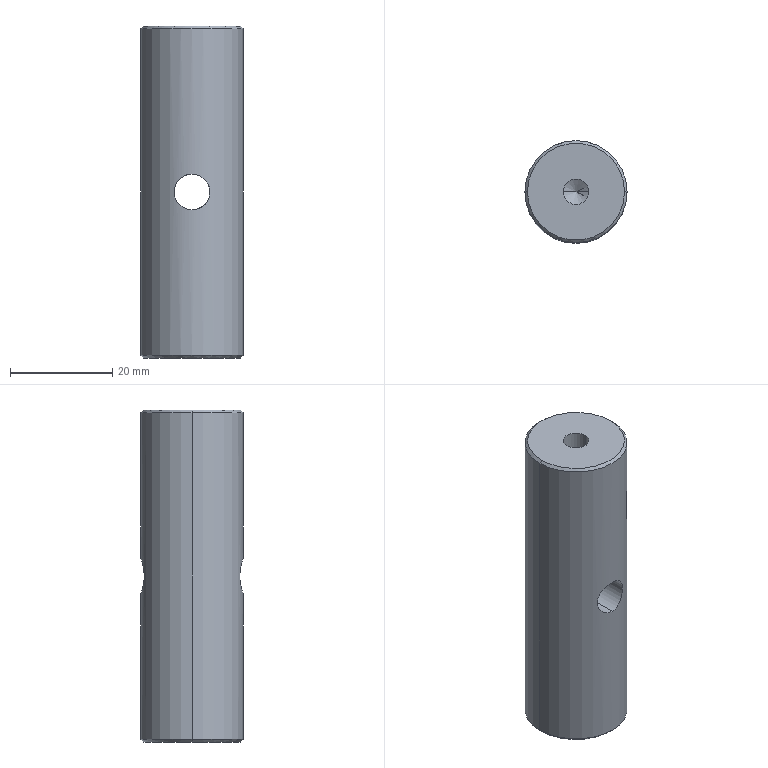Part | SolidWorks | features HoleWzd 2, Chamfer 1, Extrusion 1, ICE 1 | 1 solid | 18 faces | box 20 x 20 x 65 mm | volume 19038 mm3 | cylinder 8 | cone 8 | plane 2 | commonest cylinder face diameters 5 x4 7 x2 20 x2
STEP:
#1=CARTESIAN_POINT('',(0.,-10.,-3.5));
#2=VERTEX_POINT('',#1);
#3=CARTESIAN_POINT('',(0.,-10.,3.5));
#4=VERTEX_POINT('',#3);
#5=CARTESIAN_POINT('',(0.,-10.,-3.5));
#6=CARTESIAN_POINT('',(-0.2297,-10.,-3.5));
#7=CARTESIAN_POINT('',(-0.4614,-9.992,-3.477));
#8=CARTESIAN_POINT('',(-0.9154,-9.961,-3.386));
#9=CARTESIAN_POINT('',(-1.134,-9.938,-3.319));
#10=CARTESIAN_POINT('',(-1.557,-9.88,-3.143));
#11=CARTESIAN_POINT('',(-1.761,-9.846,-3.033));
#12=CARTESIAN_POINT('',(-2.139,-9.77,-2.78));
#13=CARTESIAN_POINT('',(-2.314,-9.73,-2.636));
#14=CARTESIAN_POINT('',(-2.637,-9.647,-2.312));
#15=CARTESIAN_POINT('',(-2.782,-9.606,-2.136));
#16=CARTESIAN_POINT('',(-3.034,-9.529,-1.759));
#17=CARTESIAN_POINT('',(-3.143,-9.494,-1.557));
#18=CARTESIAN_POINT('',(-3.32,-9.433,-1.132));
#19=CARTESIAN_POINT('',(-3.387,-9.409,-0.9133));
#20=CARTESIAN_POINT('',(-3.477,-9.376,-0.4637));
#21=CARTESIAN_POINT('',(-3.5,-9.367,-0.2298));
#22=CARTESIAN_POINT('',(-3.5,-9.368,0.2314));
#23=CARTESIAN_POINT('',(-3.477,-9.376,0.46));
#24=CARTESIAN_POINT('',(-3.387,-9.409,0.9131));
#25=CARTESIAN_POINT('',(-3.319,-9.434,1.135));
#26=CARTESIAN_POINT('',(-3.143,-9.494,1.557));
#27=CARTESIAN_POINT('',(-3.034,-9.53,1.76));
#28=CARTESIAN_POINT('',(-2.779,-9.607,2.14));
#29=CARTESIAN_POINT('',(-2.635,-9.648,2.314));
#30=CARTESIAN_POINT('',(-2.315,-9.73,2.635));
#31=CARTESIAN_POINT('',(-2.136,-9.771,2.782));
#32=CARTESIAN_POINT('',(-1.758,-9.846,3.035));
#33=CARTESIAN_POINT('',(-1.558,-9.88,3.142));
#34=CARTESIAN_POINT('',(-1.134,-9.938,3.319));
#35=CARTESIAN_POINT('',(-0.9113,-9.961,3.387));
#36=CARTESIAN_POINT('',(-0.4621,-9.992,3.477));
#37=CARTESIAN_POINT('',(-0.2332,-10.,3.5));
#38=CARTESIAN_POINT('',(0.,-10.,3.5));
#39=B_SPLINE_CURVE_WITH_KNOTS('',3,(#5,#6,#7,#8,#9,#10,#11,#12,#13,#14,#15,#16,#17,#18,#19,#20,#21,#22,#23,#24,#25,#26,#27,#28,#29,#30,#31,#32,#33,#34,#35,#36,#37,#38),.UNSPECIFIED.,.F.,.F.,(4,2,2,2,2,2,2,2,2,2,2,2,2,2,2,2,4),(0.01103,0.01172,0.01241,0.0131,0.01379,0.01448,0.01517,0.01586,0.01654,0.01723,0.01792,0.01861,0.0193,0.01999,0.02068,0.02137,0.02206),.UNSPECIFIED.);
#40=EDGE_CURVE('',#2,#4,#39,.T.);
#41=ORIENTED_EDGE('',*,*,#40,.F.);
#42=CARTESIAN_POINT('',(0.,10.,-3.5));
#43=VERTEX_POINT('',#42);
#44=CARTESIAN_POINT('',(0.,-10.,-3.5));
#45=DIRECTION('',(0.,1.,0.));
#46=VECTOR('',#45,1000.);
#47=LINE('',#44,#46);
#48=EDGE_CURVE('',#2,#43,#47,.T.);
#49=ORIENTED_EDGE('',*,*,#48,.T.);
#50=CARTESIAN_POINT('',(0.,10.,3.5));
#51=VERTEX_POINT('',#50);
#52=CARTESIAN_POINT('',(0.,10.,3.5));
#53=CARTESIAN_POINT('',(-0.2332,10.,3.5));
#54=CARTESIAN_POINT('',(-0.4622,9.992,3.477));
#55=CARTESIAN_POINT('',(-0.9122,9.961,3.387));
#56=CARTESIAN_POINT('',(-1.136,9.938,3.319));
#57=CARTESIAN_POINT('',(-1.559,9.88,3.142));
#58=CARTESIAN_POINT('',(-1.759,9.846,3.034));
#59=CARTESIAN_POINT('',(-2.138,9.771,2.78));
#60=CARTESIAN_POINT('',(-2.316,9.729,2.634));
#61=CARTESIAN_POINT('',(-2.796,9.607,2.153));
#62=CARTESIAN_POINT('',(-3.056,9.523,1.766));
#63=CARTESIAN_POINT('',(-3.318,9.434,1.136));
#64=CARTESIAN_POINT('',(-3.387,9.409,0.9132));
#65=CARTESIAN_POINT('',(-3.477,9.376,0.4605));
#66=CARTESIAN_POINT('',(-3.5,9.368,0.2322));
#67=CARTESIAN_POINT('',(-3.5,9.367,-0.2286));
#68=CARTESIAN_POINT('',(-3.477,9.376,-0.4626));
#69=CARTESIAN_POINT('',(-3.387,9.409,-0.9131));
#70=CARTESIAN_POINT('',(-3.32,9.433,-1.132));
#71=CARTESIAN_POINT('',(-3.142,9.494,-1.558));
#72=CARTESIAN_POINT('',(-3.034,9.53,-1.76));
#73=CARTESIAN_POINT('',(-2.781,9.606,-2.137));
#74=CARTESIAN_POINT('',(-2.635,9.648,-2.315));
#75=CARTESIAN_POINT('',(-2.313,9.73,-2.637));
#76=CARTESIAN_POINT('',(-2.138,9.771,-2.78));
#77=CARTESIAN_POINT('',(-1.76,9.846,-3.034));
#78=CARTESIAN_POINT('',(-1.555,9.881,-3.144));
#79=CARTESIAN_POINT('',(-1.134,9.938,-3.319));
#80=CARTESIAN_POINT('',(-0.9154,9.961,-3.386));
#81=CARTESIAN_POINT('',(-0.4616,9.992,-3.477));
#82=CARTESIAN_POINT('',(-0.2297,10.,-3.5));
#83=CARTESIAN_POINT('',(0.,10.,-3.5));
#84=B_SPLINE_CURVE_WITH_KNOTS('',3,(#52,#53,#54,#55,#56,#57,#58,#59,#60,#61,#62,#63,#64,#65,#66,#67,#68,#69,#70,#71,#72,#73,#74,#75,#76,#77,#78,#79,#80,#81,#82,#83),.UNSPECIFIED.,.F.,.F.,(4,2,2,2,2,2,2,2,2,2,2,2,2,2,2,4),(0.,0.0006894,0.001379,0.002068,0.002758,0.004136,0.004826,0.005515,0.006205,0.006894,0.007584,0.008273,0.008962,0.009652,0.01034,0.01103),.UNSPECIFIED.);
#85=EDGE_CURVE('',#51,#43,#84,.T.);
#86=ORIENTED_EDGE('',*,*,#85,.F.);
#87=CARTESIAN_POINT('',(0.,-10.,3.5));
#88=DIRECTION('',(0.,1.,0.));
#89=VECTOR('',#88,1000.);
#90=LINE('',#87,#89);
#91=EDGE_CURVE('',#4,#51,#90,.T.);
#92=ORIENTED_EDGE('',*,*,#91,.F.);
#93=EDGE_LOOP('',(#41,#49,#86,#92));
#94=FACE_OUTER_BOUND('',#93,.T.);
#95=CARTESIAN_POINT('',(0.,-10.,0.));
#96=DIRECTION('',(0.,1.,0.));
#97=DIRECTION('',(0.,0.,1.));
#98=AXIS2_PLACEMENT_3D('',#95,#96,#97);
#99=CYLINDRICAL_SURFACE('',#98,3.5);
#100=ADVANCED_FACE('',(#94),#99,.F.);
#101=CARTESIAN_POINT('',(2.5,0.,-17.5));
#102=VERTEX_POINT('',#101);
#103=CARTESIAN_POINT('',(-2.5,0.,-17.5));
#104=VERTEX_POINT('',#103);
#105=CARTESIAN_POINT('',(0.,0.,-17.5));
#106=DIRECTION('',(0.,0.,-1.));
#107=DIRECTION('',(-1.,0.,0.));
#108=AXIS2_PLACEMENT_3D('',#105,#106,#107);
#109=CIRCLE('',#108,2.5);
#110=EDGE_CURVE('',#102,#104,#109,.T.);
#111=ORIENTED_EDGE('',*,*,#110,.F.);
#112=CARTESIAN_POINT('',(2.5,0.,-32.5));
#113=VERTEX_POINT('',#112);
#114=CARTESIAN_POINT('',(2.5,0.,-32.5));
#115=DIRECTION('',(0.,0.,-1.));
#116=VECTOR('',#115,1000.);
#117=LINE('',#114,#116);
#118=EDGE_CURVE('',#102,#113,#117,.T.);
#119=ORIENTED_EDGE('',*,*,#118,.T.);
#120=CARTESIAN_POINT('',(-2.5,0.,-32.5));
#121=VERTEX_POINT('',#120);
#122=CARTESIAN_POINT('',(0.,0.,-32.5));
#123=DIRECTION('',(0.,0.,-1.));
#124=DIRECTION('',(-1.,0.,0.));
#125=AXIS2_PLACEMENT_3D('',#122,#123,#124);
#126=CIRCLE('',#125,2.5);
#127=EDGE_CURVE('',#113,#121,#126,.T.);
#128=ORIENTED_EDGE('',*,*,#127,.T.);
#129=CARTESIAN_POINT('',(-2.5,0.,-32.5));
#130=DIRECTION('',(0.,0.,-1.));
#131=VECTOR('',#130,1000.);
#132=LINE('',#129,#131);
#133=EDGE_CURVE('',#104,#121,#132,.T.);
#134=ORIENTED_EDGE('',*,*,#133,.F.);
#135=EDGE_LOOP('',(#111,#119,#128,#134));
#136=FACE_OUTER_BOUND('',#135,.T.);
#137=CARTESIAN_POINT('',(0.,0.,-32.5));
#138=DIRECTION('',(0.,0.,-1.));
#139=DIRECTION('',(-1.,0.,0.));
#140=AXIS2_PLACEMENT_3D('',#137,#138,#139);
#141=CYLINDRICAL_SURFACE('',#140,2.5);
#142=ADVANCED_FACE('',(#136),#141,.F.);
#143=CARTESIAN_POINT('',(0.,0.,-15.998));
#144=VERTEX_POINT('',#143);
#145=CARTESIAN_POINT('',(-2.5,0.,-17.5));
#146=DIRECTION('',(-0.8572,0.,-0.515));
#147=VECTOR('',#146,1000.);
#148=LINE('',#145,#147);
#149=EDGE_CURVE('',#144,#104,#148,.T.);
#150=ORIENTED_EDGE('',*,*,#149,.F.);
#151=CARTESIAN_POINT('',(2.5,0.,-17.5));
#152=DIRECTION('',(0.8572,0.,-0.515));
#153=VECTOR('',#152,1000.);
#154=LINE('',#151,#153);
#155=EDGE_CURVE('',#144,#102,#154,.T.);
#156=ORIENTED_EDGE('',*,*,#155,.T.);
#157=ORIENTED_EDGE('',*,*,#110,.T.);
#158=EDGE_LOOP('',(#150,#156,#157));
#159=FACE_OUTER_BOUND('',#158,.T.);
#160=CARTESIAN_POINT('',(0.,0.,-17.5));
#161=DIRECTION('',(0.,0.,-1.));
#162=DIRECTION('',(-1.,0.,0.));
#163=AXIS2_PLACEMENT_3D('',#160,#161,#162);
#164=CONICAL_SURFACE('',#163,2.5,1.03);
#165=ADVANCED_FACE('',(#159),#164,.F.);
#166=CARTESIAN_POINT('',(-2.5,0.,17.5));
#167=VERTEX_POINT('',#166);
#168=CARTESIAN_POINT('',(2.5,0.,17.5));
#169=VERTEX_POINT('',#168);
#170=CARTESIAN_POINT('',(0.,0.,17.5));
#171=DIRECTION('',(0.,0.,1.));
#172=DIRECTION('',(1.,0.,0.));
#173=AXIS2_PLACEMENT_3D('',#170,#171,#172);
#174=CIRCLE('',#173,2.5);
#175=EDGE_CURVE('',#167,#169,#174,.T.);
#176=ORIENTED_EDGE('',*,*,#175,.F.);
#177=CARTESIAN_POINT('',(-2.5,0.,32.5));
#178=VERTEX_POINT('',#177);
#179=CARTESIAN_POINT('',(-2.5,0.,32.5));
#180=DIRECTION('',(0.,0.,1.));
#181=VECTOR('',#180,1000.);
#182=LINE('',#179,#181);
#183=EDGE_CURVE('',#167,#178,#182,.T.);
#184=ORIENTED_EDGE('',*,*,#183,.T.);
#185=CARTESIAN_POINT('',(2.5,0.,32.5));
#186=VERTEX_POINT('',#185);
#187=CARTESIAN_POINT('',(0.,0.,32.5));
#188=DIRECTION('',(0.,0.,1.));
#189=DIRECTION('',(1.,0.,0.));
#190=AXIS2_PLACEMENT_3D('',#187,#188,#189);
#191=CIRCLE('',#190,2.5);
#192=EDGE_CURVE('',#178,#186,#191,.T.);
#193=ORIENTED_EDGE('',*,*,#192,.T.);
#194=CARTESIAN_POINT('',(2.5,0.,32.5));
#195=DIRECTION('',(0.,0.,1.));
#196=VECTOR('',#195,1000.);
#197=LINE('',#194,#196);
#198=EDGE_CURVE('',#169,#186,#197,.T.);
#199=ORIENTED_EDGE('',*,*,#198,.F.);
#200=EDGE_LOOP('',(#176,#184,#193,#199));
#201=FACE_OUTER_BOUND('',#200,.T.);
#202=CARTESIAN_POINT('',(0.,0.,32.5));
#203=DIRECTION('',(0.,0.,1.));
#204=DIRECTION('',(1.,0.,0.));
#205=AXIS2_PLACEMENT_3D('',#202,#203,#204);
#206=CYLINDRICAL_SURFACE('',#205,2.5);
#207=ADVANCED_FACE('',(#201),#206,.F.);
#208=CARTESIAN_POINT('',(0.,0.,15.998));
#209=VERTEX_POINT('',#208);
#210=CARTESIAN_POINT('',(2.5,0.,17.5));
#211=DIRECTION('',(0.8572,0.,0.515));
#212=VECTOR('',#211,1000.);
#213=LINE('',#210,#212);
#214=EDGE_CURVE('',#209,#169,#213,.T.);
#215=ORIENTED_EDGE('',*,*,#214,.F.);
#216=CARTESIAN_POINT('',(-2.5,0.,17.5));
#217=DIRECTION('',(-0.8572,0.,0.515));
#218=VECTOR('',#217,1000.);
#219=LINE('',#216,#218);
#220=EDGE_CURVE('',#209,#167,#219,.T.);
#221=ORIENTED_EDGE('',*,*,#220,.T.);
#222=ORIENTED_EDGE('',*,*,#175,.T.);
#223=EDGE_LOOP('',(#215,#221,#222));
#224=FACE_OUTER_BOUND('',#223,.T.);
#225=CARTESIAN_POINT('',(0.,0.,17.5));
#226=DIRECTION('',(0.,0.,1.));
#227=DIRECTION('',(1.,0.,0.));
#228=AXIS2_PLACEMENT_3D('',#225,#226,#227);
#229=CONICAL_SURFACE('',#228,2.5,1.03);
#230=ADVANCED_FACE('',(#224),#229,.F.);
#231=CARTESIAN_POINT('',(9.5,0.,32.5));
#232=VERTEX_POINT('',#231);
#233=CARTESIAN_POINT('',(-9.5,0.,32.5));
#234=VERTEX_POINT('',#233);
#235=CARTESIAN_POINT('',(0.,0.,32.5));
#236=DIRECTION('',(0.,0.,1.));
#237=DIRECTION('',(1.,0.,0.));
#238=AXIS2_PLACEMENT_3D('',#235,#236,#237);
#239=CIRCLE('',#238,9.5);
#240=EDGE_CURVE('',#232,#234,#239,.T.);
#241=ORIENTED_EDGE('',*,*,#240,.F.);
#242=CARTESIAN_POINT('',(10.,0.,32.));
#243=VERTEX_POINT('',#242);
#244=CARTESIAN_POINT('',(9.5,0.,32.5));
#245=DIRECTION('',(0.7071,0.,-0.7071));
#246=VECTOR('',#245,1000.);
#247=LINE('',#244,#246);
#248=EDGE_CURVE('',#232,#243,#247,.T.);
#249=ORIENTED_EDGE('',*,*,#248,.T.);
#250=CARTESIAN_POINT('',(-10.,0.,32.));
#251=VERTEX_POINT('',#250);
#252=CARTESIAN_POINT('',(0.,0.,32.));
#253=DIRECTION('',(0.,0.,-1.));
#254=DIRECTION('',(1.,0.,0.));
#255=AXIS2_PLACEMENT_3D('',#252,#253,#254);
#256=CIRCLE('',#255,10.);
#257=EDGE_CURVE('',#251,#243,#256,.T.);
#258=ORIENTED_EDGE('',*,*,#257,.F.);
#259=CARTESIAN_POINT('',(-9.5,0.,32.5));
#260=DIRECTION('',(-0.7071,0.,-0.7071));
#261=VECTOR('',#260,1000.);
#262=LINE('',#259,#261);
#263=EDGE_CURVE('',#234,#251,#262,.T.);
#264=ORIENTED_EDGE('',*,*,#263,.F.);
#265=EDGE_LOOP('',(#241,#249,#258,#264));
#266=FACE_OUTER_BOUND('',#265,.T.);
#267=CARTESIAN_POINT('',(0.,0.,32.5));
#268=DIRECTION('',(0.,0.,-1.));
#269=DIRECTION('',(-1.,0.,0.));
#270=AXIS2_PLACEMENT_3D('',#267,#268,#269);
#271=CONICAL_SURFACE('',#270,9.5,0.7854);
#272=ADVANCED_FACE('',(#266),#271,.T.);
#273=CARTESIAN_POINT('',(-9.5,0.,-32.5));
#274=VERTEX_POINT('',#273);
#275=CARTESIAN_POINT('',(9.5,0.,-32.5));
#276=VERTEX_POINT('',#275);
#277=CARTESIAN_POINT('',(0.,0.,-32.5));
#278=DIRECTION('',(0.,0.,-1.));
#279=DIRECTION('',(1.,0.,0.));
#280=AXIS2_PLACEMENT_3D('',#277,#278,#279);
#281=CIRCLE('',#280,9.5);
#282=EDGE_CURVE('',#274,#276,#281,.T.);
#283=ORIENTED_EDGE('',*,*,#282,.F.);
#284=CARTESIAN_POINT('',(-10.,0.,-32.));
#285=VERTEX_POINT('',#284);
#286=CARTESIAN_POINT('',(-10.,0.,-32.));
#287=DIRECTION('',(-0.7071,0.,0.7071));
#288=VECTOR('',#287,1000.);
#289=LINE('',#286,#288);
#290=EDGE_CURVE('',#274,#285,#289,.T.);
#291=ORIENTED_EDGE('',*,*,#290,.T.);
#292=CARTESIAN_POINT('',(10.,0.,-32.));
#293=VERTEX_POINT('',#292);
#294=CARTESIAN_POINT('',(0.,0.,-32.));
#295=DIRECTION('',(0.,0.,1.));
#296=DIRECTION('',(1.,0.,0.));
#297=AXIS2_PLACEMENT_3D('',#294,#295,#296);
#298=CIRCLE('',#297,10.);
#299=EDGE_CURVE('',#293,#285,#298,.T.);
#300=ORIENTED_EDGE('',*,*,#299,.F.);
#301=CARTESIAN_POINT('',(10.,0.,-32.));
#302=DIRECTION('',(0.7071,0.,0.7071));
#303=VECTOR('',#302,1000.);
#304=LINE('',#301,#303);
#305=EDGE_CURVE('',#276,#293,#304,.T.);
#306=ORIENTED_EDGE('',*,*,#305,.F.);
#307=EDGE_LOOP('',(#283,#291,#300,#306));
#308=FACE_OUTER_BOUND('',#307,.T.);
#309=CARTESIAN_POINT('',(0.,0.,-32.));
#310=DIRECTION('',(0.,0.,1.));
#311=DIRECTION('',(1.,0.,0.));
#312=AXIS2_PLACEMENT_3D('',#309,#310,#311);
#313=CONICAL_SURFACE('',#312,10.,0.7854);
#314=ADVANCED_FACE('',(#308),#313,.T.);
#315=ORIENTED_EDGE('',*,*,#85,.T.);
#316=CARTESIAN_POINT('',(0.,10.,-3.5));
#317=CARTESIAN_POINT('',(0.2297,10.,-3.5));
#318=CARTESIAN_POINT('',(0.4614,9.992,-3.477));
#319=CARTESIAN_POINT('',(0.9154,9.961,-3.386));
#320=CARTESIAN_POINT('',(1.134,9.938,-3.319));
#321=CARTESIAN_POINT('',(1.557,9.88,-3.143));
#322=CARTESIAN_POINT('',(1.761,9.846,-3.033));
#323=CARTESIAN_POINT('',(2.139,9.77,-2.78));
#324=CARTESIAN_POINT('',(2.314,9.73,-2.636));
#325=CARTESIAN_POINT('',(2.637,9.647,-2.312));
#326=CARTESIAN_POINT('',(2.782,9.606,-2.136));
#327=CARTESIAN_POINT('',(3.034,9.529,-1.759));
#328=CARTESIAN_POINT('',(3.143,9.494,-1.557));
#329=CARTESIAN_POINT('',(3.32,9.433,-1.132));
#330=CARTESIAN_POINT('',(3.387,9.409,-0.9133));
#331=CARTESIAN_POINT('',(3.477,9.376,-0.4637));
#332=CARTESIAN_POINT('',(3.5,9.367,-0.2298));
#333=CARTESIAN_POINT('',(3.5,9.368,0.2314));
#334=CARTESIAN_POINT('',(3.477,9.376,0.46));
#335=CARTESIAN_POINT('',(3.387,9.409,0.9131));
#336=CARTESIAN_POINT('',(3.319,9.434,1.135));
#337=CARTESIAN_POINT('',(3.143,9.494,1.557));
#338=CARTESIAN_POINT('',(3.034,9.53,1.76));
#339=CARTESIAN_POINT('',(2.779,9.607,2.14));
#340=CARTESIAN_POINT('',(2.635,9.648,2.314));
#341=CARTESIAN_POINT('',(2.315,9.73,2.635));
#342=CARTESIAN_POINT('',(2.136,9.771,2.782));
#343=CARTESIAN_POINT('',(1.758,9.846,3.035));
#344=CARTESIAN_POINT('',(1.558,9.88,3.142));
#345=CARTESIAN_POINT('',(1.134,9.938,3.319));
#346=CARTESIAN_POINT('',(0.9113,9.961,3.387));
#347=CARTESIAN_POINT('',(0.4621,9.992,3.477));
#348=CARTESIAN_POINT('',(0.2332,10.,3.5));
#349=CARTESIAN_POINT('',(0.,10.,3.5));
#350=B_SPLINE_CURVE_WITH_KNOTS('',3,(#316,#317,#318,#319,#320,#321,#322,#323,#324,#325,#326,#327,#328,#329,#330,#331,#332,#333,#334,#335,#336,#337,#338,#339,#340,#341,#342,#343,#344,#345,#346,#347,#348,#349),.UNSPECIFIED.,.F.,.F.,(4,2,2,2,2,2,2,2,2,2,2,2,2,2,2,2,4),(0.01103,0.01172,0.01241,0.0131,0.01379,0.01448,0.01517,0.01586,0.01654,0.01723,0.01792,0.01861,0.0193,0.01999,0.02068,0.02137,0.02206),.UNSPECIFIED.);
#351=EDGE_CURVE('',#43,#51,#350,.T.);
#352=ORIENTED_EDGE('',*,*,#351,.T.);
#353=EDGE_LOOP('',(#315,#352));
#354=FACE_BOUND('',#353,.T.);
#355=ORIENTED_EDGE('',*,*,#257,.T.);
#356=CARTESIAN_POINT('',(10.,0.,32.5));
#357=DIRECTION('',(0.,0.,-1.));
#358=VECTOR('',#357,1000.);
#359=LINE('',#356,#358);
#360=EDGE_CURVE('',#243,#293,#359,.T.);
#361=ORIENTED_EDGE('',*,*,#360,.T.);
#362=ORIENTED_EDGE('',*,*,#299,.T.);
#363=CARTESIAN_POINT('',(-10.,0.,32.5));
#364=DIRECTION('',(0.,0.,-1.));
#365=VECTOR('',#364,1000.);
#366=LINE('',#363,#365);
#367=EDGE_CURVE('',#251,#285,#366,.T.);
#368=ORIENTED_EDGE('',*,*,#367,.F.);
#369=EDGE_LOOP('',(#355,#361,#362,#368));
#370=FACE_OUTER_BOUND('',#369,.T.);
#371=CARTESIAN_POINT('',(0.,0.,32.5));
#372=DIRECTION('',(0.,0.,-1.));
#373=DIRECTION('',(-1.,0.,0.));
#374=AXIS2_PLACEMENT_3D('',#371,#372,#373);
#375=CYLINDRICAL_SURFACE('',#374,10.);
#376=ADVANCED_FACE('',(#354,#370),#375,.T.);
#377=ORIENTED_EDGE('',*,*,#360,.F.);
#378=CARTESIAN_POINT('',(0.,0.,32.));
#379=DIRECTION('',(0.,0.,-1.));
#380=DIRECTION('',(1.,0.,0.));
#381=AXIS2_PLACEMENT_3D('',#378,#379,#380);
#382=CIRCLE('',#381,10.);
#383=EDGE_CURVE('',#243,#251,#382,.T.);
#384=ORIENTED_EDGE('',*,*,#383,.T.);
#385=ORIENTED_EDGE('',*,*,#367,.T.);
#386=CARTESIAN_POINT('',(0.,0.,-32.));
#387=DIRECTION('',(0.,0.,1.));
#388=DIRECTION('',(1.,0.,0.));
#389=AXIS2_PLACEMENT_3D('',#386,#387,#388);
#390=CIRCLE('',#389,10.);
#391=EDGE_CURVE('',#285,#293,#390,.T.);
#392=ORIENTED_EDGE('',*,*,#391,.T.);
#393=EDGE_LOOP('',(#377,#384,#385,#392));
#394=FACE_OUTER_BOUND('',#393,.T.);
#395=CARTESIAN_POINT('',(0.,-10.,3.5));
#396=CARTESIAN_POINT('',(0.2332,-10.,3.5));
#397=CARTESIAN_POINT('',(0.4622,-9.992,3.477));
#398=CARTESIAN_POINT('',(0.9122,-9.961,3.387));
#399=CARTESIAN_POINT('',(1.136,-9.938,3.319));
#400=CARTESIAN_POINT('',(1.559,-9.88,3.142));
#401=CARTESIAN_POINT('',(1.759,-9.846,3.034));
#402=CARTESIAN_POINT('',(2.138,-9.771,2.78));
#403=CARTESIAN_POINT('',(2.316,-9.729,2.634));
#404=CARTESIAN_POINT('',(2.796,-9.607,2.153));
#405=CARTESIAN_POINT('',(3.056,-9.523,1.766));
#406=CARTESIAN_POINT('',(3.318,-9.434,1.136));
#407=CARTESIAN_POINT('',(3.387,-9.409,0.9132));
#408=CARTESIAN_POINT('',(3.477,-9.376,0.4605));
#409=CARTESIAN_POINT('',(3.5,-9.368,0.2322));
#410=CARTESIAN_POINT('',(3.5,-9.367,-0.2286));
#411=CARTESIAN_POINT('',(3.477,-9.376,-0.4626));
#412=CARTESIAN_POINT('',(3.387,-9.409,-0.9131));
#413=CARTESIAN_POINT('',(3.32,-9.433,-1.132));
#414=CARTESIAN_POINT('',(3.142,-9.494,-1.558));
#415=CARTESIAN_POINT('',(3.034,-9.53,-1.76));
#416=CARTESIAN_POINT('',(2.781,-9.606,-2.137));
#417=CARTESIAN_POINT('',(2.635,-9.648,-2.315));
#418=CARTESIAN_POINT('',(2.313,-9.73,-2.637));
#419=CARTESIAN_POINT('',(2.138,-9.771,-2.78));
#420=CARTESIAN_POINT('',(1.76,-9.846,-3.034));
#421=CARTESIAN_POINT('',(1.555,-9.881,-3.144));
#422=CARTESIAN_POINT('',(1.134,-9.938,-3.319));
#423=CARTESIAN_POINT('',(0.9154,-9.961,-3.386));
#424=CARTESIAN_POINT('',(0.4616,-9.992,-3.477));
#425=CARTESIAN_POINT('',(0.2297,-10.,-3.5));
#426=CARTESIAN_POINT('',(0.,-10.,-3.5));
#427=B_SPLINE_CURVE_WITH_KNOTS('',3,(#395,#396,#397,#398,#399,#400,#401,#402,#403,#404,#405,#406,#407,#408,#409,#410,#411,#412,#413,#414,#415,#416,#417,#418,#419,#420,#421,#422,#423,#424,#425,#426),.UNSPECIFIED.,.F.,.F.,(4,2,2,2,2,2,2,2,2,2,2,2,2,2,2,4),(0.,0.0006894,0.001379,0.002068,0.002758,0.004136,0.004826,0.005515,0.006205,0.006894,0.007584,0.008273,0.008962,0.009652,0.01034,0.01103),.UNSPECIFIED.);
#428=EDGE_CURVE('',#4,#2,#427,.T.);
#429=ORIENTED_EDGE('',*,*,#428,.T.);
#430=ORIENTED_EDGE('',*,*,#40,.T.);
#431=EDGE_LOOP('',(#429,#430));
#432=FACE_BOUND('',#431,.T.);
#433=CARTESIAN_POINT('',(0.,0.,32.5));
#434=DIRECTION('',(0.,0.,-1.));
#435=DIRECTION('',(-1.,0.,0.));
#436=AXIS2_PLACEMENT_3D('',#433,#434,#435);
#437=CYLINDRICAL_SURFACE('',#436,10.);
#438=ADVANCED_FACE('',(#394,#432),#437,.T.);
#439=CARTESIAN_POINT('',(0.,0.,32.5));
#440=DIRECTION('',(0.,0.,1.));
#441=DIRECTION('',(1.,0.,0.));
#442=AXIS2_PLACEMENT_3D('',#439,#440,#441);
#443=CIRCLE('',#442,2.5);
#444=EDGE_CURVE('',#186,#178,#443,.T.);
#445=ORIENTED_EDGE('',*,*,#444,.F.);
#446=ORIENTED_EDGE('',*,*,#192,.F.);
#447=EDGE_LOOP('',(#445,#446));
#448=FACE_BOUND('',#447,.T.);
#449=CARTESIAN_POINT('',(0.,0.,32.5));
#450=DIRECTION('',(0.,0.,1.));
#451=DIRECTION('',(1.,0.,0.));
#452=AXIS2_PLACEMENT_3D('',#449,#450,#451);
#453=CIRCLE('',#452,9.5);
#454=EDGE_CURVE('',#234,#232,#453,.T.);
#455=ORIENTED_EDGE('',*,*,#454,.T.);
#456=ORIENTED_EDGE('',*,*,#240,.T.);
#457=EDGE_LOOP('',(#455,#456));
#458=FACE_OUTER_BOUND('',#457,.T.);
#459=CARTESIAN_POINT('',(0.,0.,32.5));
#460=DIRECTION('',(0.,0.,1.));
#461=DIRECTION('',(1.,0.,0.));
#462=AXIS2_PLACEMENT_3D('',#459,#460,#461);
#463=PLANE('',#462);
#464=ADVANCED_FACE('',(#448,#458),#463,.T.);
#465=CARTESIAN_POINT('',(0.,0.,-32.5));
#466=DIRECTION('',(0.,0.,-1.));
#467=DIRECTION('',(-1.,0.,0.));
#468=AXIS2_PLACEMENT_3D('',#465,#466,#467);
#469=CIRCLE('',#468,2.5);
#470=EDGE_CURVE('',#121,#113,#469,.T.);
#471=ORIENTED_EDGE('',*,*,#470,.F.);
#472=ORIENTED_EDGE('',*,*,#127,.F.);
#473=EDGE_LOOP('',(#471,#472));
#474=FACE_BOUND('',#473,.T.);
#475=CARTESIAN_POINT('',(0.,0.,-32.5));
#476=DIRECTION('',(0.,0.,-1.));
#477=DIRECTION('',(1.,0.,0.));
#478=AXIS2_PLACEMENT_3D('',#475,#476,#477);
#479=CIRCLE('',#478,9.5);
#480=EDGE_CURVE('',#276,#274,#479,.T.);
#481=ORIENTED_EDGE('',*,*,#480,.T.);
#482=ORIENTED_EDGE('',*,*,#282,.T.);
#483=EDGE_LOOP('',(#481,#482));
#484=FACE_OUTER_BOUND('',#483,.T.);
#485=CARTESIAN_POINT('',(0.,0.,-32.5));
#486=DIRECTION('',(0.,0.,1.));
#487=DIRECTION('',(1.,0.,0.));
#488=AXIS2_PLACEMENT_3D('',#485,#486,#487);
#489=PLANE('',#488);
#490=ADVANCED_FACE('',(#474,#484),#489,.F.);
#491=ORIENTED_EDGE('',*,*,#290,.F.);
#492=ORIENTED_EDGE('',*,*,#480,.F.);
#493=ORIENTED_EDGE('',*,*,#305,.T.);
#494=ORIENTED_EDGE('',*,*,#391,.F.);
#495=EDGE_LOOP('',(#491,#492,#493,#494));
#496=FACE_OUTER_BOUND('',#495,.T.);
#497=CARTESIAN_POINT('',(0.,0.,-32.));
#498=DIRECTION('',(0.,0.,1.));
#499=DIRECTION('',(1.,0.,0.));
#500=AXIS2_PLACEMENT_3D('',#497,#498,#499);
#501=CONICAL_SURFACE('',#500,10.,0.7854);
#502=ADVANCED_FACE('',(#496),#501,.T.);
#503=ORIENTED_EDGE('',*,*,#248,.F.);
#504=ORIENTED_EDGE('',*,*,#454,.F.);
#505=ORIENTED_EDGE('',*,*,#263,.T.);
#506=ORIENTED_EDGE('',*,*,#383,.F.);
#507=EDGE_LOOP('',(#503,#504,#505,#506));
#508=FACE_OUTER_BOUND('',#507,.T.);
#509=CARTESIAN_POINT('',(0.,0.,32.5));
#510=DIRECTION('',(0.,0.,-1.));
#511=DIRECTION('',(-1.,0.,0.));
#512=AXIS2_PLACEMENT_3D('',#509,#510,#511);
#513=CONICAL_SURFACE('',#512,9.5,0.7854);
#514=ADVANCED_FACE('',(#508),#513,.T.);
#515=ORIENTED_EDGE('',*,*,#220,.F.);
#516=ORIENTED_EDGE('',*,*,#214,.T.);
#517=CARTESIAN_POINT('',(0.,0.,17.5));
#518=DIRECTION('',(0.,0.,1.));
#519=DIRECTION('',(1.,0.,0.));
#520=AXIS2_PLACEMENT_3D('',#517,#518,#519);
#521=CIRCLE('',#520,2.5);
#522=EDGE_CURVE('',#169,#167,#521,.T.);
#523=ORIENTED_EDGE('',*,*,#522,.T.);
#524=EDGE_LOOP('',(#515,#516,#523));
#525=FACE_OUTER_BOUND('',#524,.T.);
#526=CARTESIAN_POINT('',(0.,0.,17.5));
#527=DIRECTION('',(0.,0.,1.));
#528=DIRECTION('',(1.,0.,0.));
#529=AXIS2_PLACEMENT_3D('',#526,#527,#528);
#530=CONICAL_SURFACE('',#529,2.5,1.03);
#531=ADVANCED_FACE('',(#525),#530,.F.);
#532=ORIENTED_EDGE('',*,*,#183,.F.);
#533=ORIENTED_EDGE('',*,*,#522,.F.);
#534=ORIENTED_EDGE('',*,*,#198,.T.);
#535=ORIENTED_EDGE('',*,*,#444,.T.);
#536=EDGE_LOOP('',(#532,#533,#534,#535));
#537=FACE_OUTER_BOUND('',#536,.T.);
#538=CARTESIAN_POINT('',(0.,0.,32.5));
#539=DIRECTION('',(0.,0.,1.));
#540=DIRECTION('',(1.,0.,0.));
#541=AXIS2_PLACEMENT_3D('',#538,#539,#540);
#542=CYLINDRICAL_SURFACE('',#541,2.5);
#543=ADVANCED_FACE('',(#537),#542,.F.);
#544=ORIENTED_EDGE('',*,*,#155,.F.);
#545=ORIENTED_EDGE('',*,*,#149,.T.);
#546=CARTESIAN_POINT('',(0.,0.,-17.5));
#547=DIRECTION('',(0.,0.,-1.));
#548=DIRECTION('',(-1.,0.,0.));
#549=AXIS2_PLACEMENT_3D('',#546,#547,#548);
#550=CIRCLE('',#549,2.5);
#551=EDGE_CURVE('',#104,#102,#550,.T.);
#552=ORIENTED_EDGE('',*,*,#551,.T.);
#553=EDGE_LOOP('',(#544,#545,#552));
#554=FACE_OUTER_BOUND('',#553,.T.);
#555=CARTESIAN_POINT('',(0.,0.,-17.5));
#556=DIRECTION('',(0.,0.,-1.));
#557=DIRECTION('',(-1.,0.,0.));
#558=AXIS2_PLACEMENT_3D('',#555,#556,#557);
#559=CONICAL_SURFACE('',#558,2.5,1.03);
#560=ADVANCED_FACE('',(#554),#559,.F.);
#561=ORIENTED_EDGE('',*,*,#118,.F.);
#562=ORIENTED_EDGE('',*,*,#551,.F.);
#563=ORIENTED_EDGE('',*,*,#133,.T.);
#564=ORIENTED_EDGE('',*,*,#470,.T.);
#565=EDGE_LOOP('',(#561,#562,#563,#564));
#566=FACE_OUTER_BOUND('',#565,.T.);
#567=CARTESIAN_POINT('',(0.,0.,-32.5));
#568=DIRECTION('',(0.,0.,-1.));
#569=DIRECTION('',(-1.,0.,0.));
#570=AXIS2_PLACEMENT_3D('',#567,#568,#569);
#571=CYLINDRICAL_SURFACE('',#570,2.5);
#572=ADVANCED_FACE('',(#566),#571,.F.);
#573=ORIENTED_EDGE('',*,*,#48,.F.);
#574=ORIENTED_EDGE('',*,*,#428,.F.);
#575=ORIENTED_EDGE('',*,*,#91,.T.);
#576=ORIENTED_EDGE('',*,*,#351,.F.);
#577=EDGE_LOOP('',(#573,#574,#575,#576));
#578=FACE_OUTER_BOUND('',#577,.T.);
#579=CARTESIAN_POINT('',(0.,-10.,0.));
#580=DIRECTION('',(0.,1.,0.));
#581=DIRECTION('',(0.,0.,1.));
#582=AXIS2_PLACEMENT_3D('',#579,#580,#581);
#583=CYLINDRICAL_SURFACE('',#582,3.5);
#584=ADVANCED_FACE('',(#578),#583,.F.);
#585=CLOSED_SHELL('',(#100,#142,#165,#207,#230,#272,#314,#376,#438,#464,#490,#502,#514,#531,#543,#560,#572,#584));
#586=MANIFOLD_SOLID_BREP('',#585);
#587=CARTESIAN_POINT('',(0.,0.,0.));
#588=DIRECTION('',(0.,0.,1.));
#589=DIRECTION('',(1.,0.,0.));
#590=AXIS2_PLACEMENT_3D('',#587,#588,#589);
#591=(LENGTH_UNIT()NAMED_UNIT(*)SI_UNIT(.MILLI.,.METRE.));
#592=UNCERTAINTY_MEASURE_WITH_UNIT(LENGTH_MEASURE(0.00001),#591,'','');
#593=(NAMED_UNIT(*)PLANE_ANGLE_UNIT()SI_UNIT($,.RADIAN.));
#594=(NAMED_UNIT(*)SI_UNIT($,.STERADIAN.)SOLID_ANGLE_UNIT());
#595=(GEOMETRIC_REPRESENTATION_CONTEXT(3)GLOBAL_UNCERTAINTY_ASSIGNED_CONTEXT((#592))GLOBAL_UNIT_ASSIGNED_CONTEXT((#591,#593,#594))REPRESENTATION_CONTEXT('',''));
#596=ADVANCED_BREP_SHAPE_REPRESENTATION('',(#586,#590),#595);